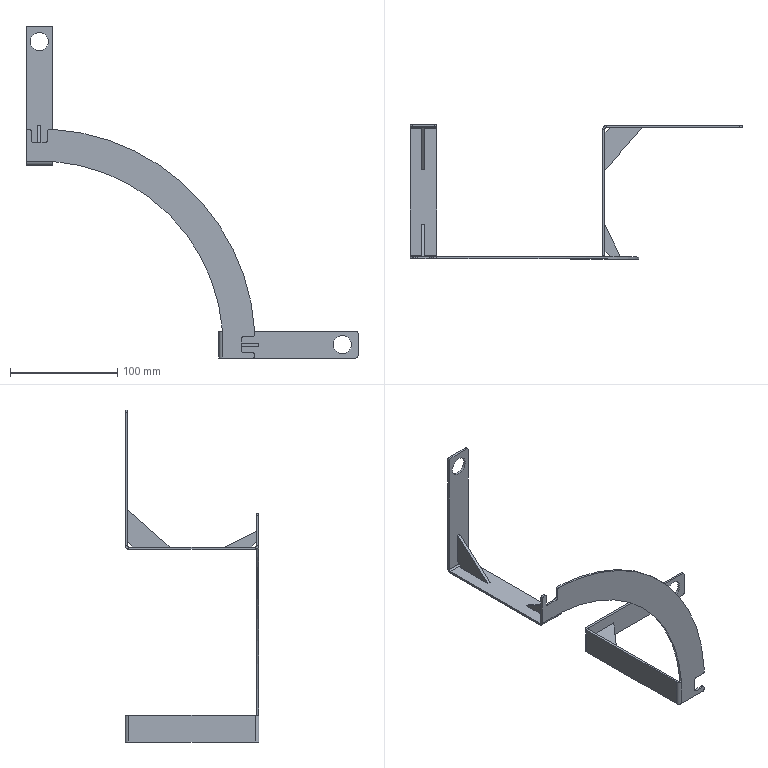Part | STEP file | 17-Detection plate_default<machined> | 5 solids | 94 faces | box 310.044 x 125 x 310.044 mm | volume 48050 mm3 | plane 64 | cylinder 30 | commonest cylinder face diameters 4 x16 3 x4 7 x4 17 x4 343 x1 403 x1